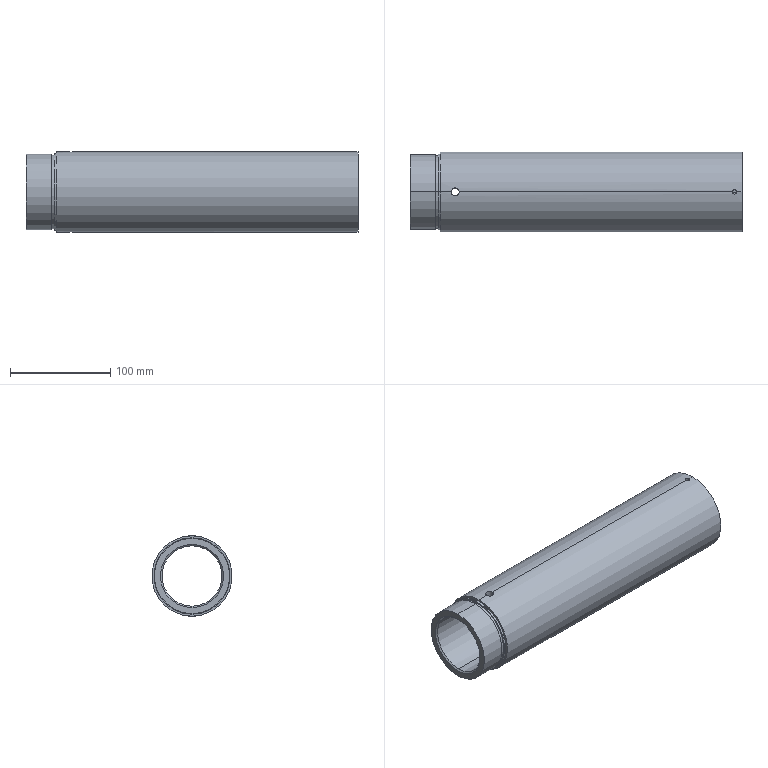Part | SolidWorks | features ICE 3, Chamfer 2, HoleWzd 1, Revolution 1 | 1 solid | 28 faces | box 330.5 x 80 x 80 mm | volume 682443 mm3 | cylinder 18 | plane 6 | cone 4 | commonest cylinder face diameters 8 x4 4.2 x2 60 x2 65 x2 73 x2 75 x2
STEP:
#1=CARTESIAN_POINT('',(320.9,0.,40.));
#2=VERTEX_POINT('',#1);
#3=CARTESIAN_POINT('',(325.1,0.,40.));
#4=VERTEX_POINT('',#3);
#5=CARTESIAN_POINT('',(320.9,0.,40.));
#6=CARTESIAN_POINT('',(320.9,-0.1388,40.));
#7=CARTESIAN_POINT('',(320.914,-0.2752,39.999));
#8=CARTESIAN_POINT('',(320.967,-0.5437,39.997));
#9=CARTESIAN_POINT('',(321.007,-0.6771,39.994));
#10=CARTESIAN_POINT('',(321.113,-0.9314,39.989));
#11=CARTESIAN_POINT('',(321.177,-1.052,39.986));
#12=CARTESIAN_POINT('',(321.33,-1.28,39.98));
#13=CARTESIAN_POINT('',(321.418,-1.388,39.976));
#14=CARTESIAN_POINT('',(321.709,-1.679,39.965));
#15=CARTESIAN_POINT('',(321.943,-1.835,39.958));
#16=CARTESIAN_POINT('',(322.449,-2.045,39.948));
#17=CARTESIAN_POINT('',(322.725,-2.1,39.945));
#18=CARTESIAN_POINT('',(323.136,-2.1,39.945));
#19=CARTESIAN_POINT('',(323.275,-2.086,39.946));
#20=CARTESIAN_POINT('',(323.545,-2.033,39.948));
#21=CARTESIAN_POINT('',(323.676,-1.993,39.95));
#22=CARTESIAN_POINT('',(323.93,-1.888,39.955));
#23=CARTESIAN_POINT('',(324.053,-1.822,39.959));
#24=CARTESIAN_POINT('',(324.28,-1.67,39.965));
#25=CARTESIAN_POINT('',(324.387,-1.583,39.969));
#26=CARTESIAN_POINT('',(324.583,-1.387,39.976));
#27=CARTESIAN_POINT('',(324.67,-1.281,39.98));
#28=CARTESIAN_POINT('',(324.822,-1.054,39.986));
#29=CARTESIAN_POINT('',(324.887,-0.9308,39.989));
#30=CARTESIAN_POINT('',(324.993,-0.6763,39.994));
#31=CARTESIAN_POINT('',(325.033,-0.5454,39.997));
#32=CARTESIAN_POINT('',(325.086,-0.2763,39.999));
#33=CARTESIAN_POINT('',(325.1,-0.1371,40.));
#34=CARTESIAN_POINT('',(325.1,0.,40.));
#35=B_SPLINE_CURVE_WITH_KNOTS('',3,(#5,#6,#7,#8,#9,#10,#11,#12,#13,#14,#15,#16,#17,#18,#19,#20,#21,#22,#23,#24,#25,#26,#27,#28,#29,#30,#31,#32,#33,#34),.UNSPECIFIED.,.F.,.F.,(4,2,2,2,2,2,2,2,2,2,2,2,2,2,4),(0.,0.0004104,0.0008208,0.001231,0.001642,0.002463,0.003283,0.003694,0.004104,0.004515,0.004925,0.005335,0.005746,0.006156,0.006567),.UNSPECIFIED.);
#36=EDGE_CURVE('',#2,#4,#35,.T.);
#37=ORIENTED_EDGE('',*,*,#36,.T.);
#38=CARTESIAN_POINT('',(325.1,0.,32.5));
#39=VERTEX_POINT('',#38);
#40=CARTESIAN_POINT('',(325.1,0.,0.));
#41=DIRECTION('',(0.,0.,-1.));
#42=VECTOR('',#41,1000.);
#43=LINE('',#40,#42);
#44=EDGE_CURVE('',#4,#39,#43,.T.);
#45=ORIENTED_EDGE('',*,*,#44,.T.);
#46=CARTESIAN_POINT('',(320.9,0.,32.5));
#47=VERTEX_POINT('',#46);
#48=CARTESIAN_POINT('',(320.9,0.,32.5));
#49=CARTESIAN_POINT('',(320.9,-0.1388,32.5));
#50=CARTESIAN_POINT('',(320.914,-0.2753,32.499));
#51=CARTESIAN_POINT('',(320.967,-0.5437,32.496));
#52=CARTESIAN_POINT('',(321.007,-0.6771,32.493));
#53=CARTESIAN_POINT('',(321.113,-0.9314,32.487));
#54=CARTESIAN_POINT('',(321.177,-1.052,32.483));
#55=CARTESIAN_POINT('',(321.33,-1.28,32.475));
#56=CARTESIAN_POINT('',(321.418,-1.388,32.47));
#57=CARTESIAN_POINT('',(321.709,-1.679,32.457));
#58=CARTESIAN_POINT('',(321.943,-1.835,32.448));
#59=CARTESIAN_POINT('',(322.449,-2.045,32.436));
#60=CARTESIAN_POINT('',(322.725,-2.1,32.432));
#61=CARTESIAN_POINT('',(323.136,-2.1,32.432));
#62=CARTESIAN_POINT('',(323.275,-2.086,32.433));
#63=CARTESIAN_POINT('',(323.545,-2.033,32.436));
#64=CARTESIAN_POINT('',(323.676,-1.993,32.439));
#65=CARTESIAN_POINT('',(323.93,-1.888,32.445));
#66=CARTESIAN_POINT('',(324.053,-1.822,32.449));
#67=CARTESIAN_POINT('',(324.281,-1.67,32.457));
#68=CARTESIAN_POINT('',(324.387,-1.583,32.462));
#69=CARTESIAN_POINT('',(324.583,-1.387,32.471));
#70=CARTESIAN_POINT('',(324.67,-1.281,32.475));
#71=CARTESIAN_POINT('',(324.822,-1.054,32.483));
#72=CARTESIAN_POINT('',(324.887,-0.9308,32.487));
#73=CARTESIAN_POINT('',(324.993,-0.6764,32.493));
#74=CARTESIAN_POINT('',(325.033,-0.5455,32.496));
#75=CARTESIAN_POINT('',(325.086,-0.2763,32.499));
#76=CARTESIAN_POINT('',(325.1,-0.1371,32.5));
#77=CARTESIAN_POINT('',(325.1,0.,32.5));
#78=B_SPLINE_CURVE_WITH_KNOTS('',3,(#48,#49,#50,#51,#52,#53,#54,#55,#56,#57,#58,#59,#60,#61,#62,#63,#64,#65,#66,#67,#68,#69,#70,#71,#72,#73,#74,#75,#76,#77),.UNSPECIFIED.,.F.,.F.,(4,2,2,2,2,2,2,2,2,2,2,2,2,2,4),(0.,0.0004105,0.0008209,0.001231,0.001642,0.002463,0.003284,0.003694,0.004105,0.004515,0.004925,0.005336,0.005746,0.006157,0.006567),.UNSPECIFIED.);
#79=EDGE_CURVE('',#47,#39,#78,.T.);
#80=ORIENTED_EDGE('',*,*,#79,.F.);
#81=CARTESIAN_POINT('',(320.9,0.,0.));
#82=DIRECTION('',(0.,0.,-1.));
#83=VECTOR('',#82,1000.);
#84=LINE('',#81,#83);
#85=EDGE_CURVE('',#2,#47,#84,.T.);
#86=ORIENTED_EDGE('',*,*,#85,.F.);
#87=EDGE_LOOP('',(#37,#45,#80,#86));
#88=FACE_OUTER_BOUND('',#87,.T.);
#89=CARTESIAN_POINT('',(323.,0.,0.));
#90=DIRECTION('',(0.,0.,-1.));
#91=DIRECTION('',(-1.,0.,0.));
#92=AXIS2_PLACEMENT_3D('',#89,#90,#91);
#93=CYLINDRICAL_SURFACE('',#92,2.1);
#94=ADVANCED_FACE('',(#88),#93,.F.);
#95=CARTESIAN_POINT('',(49.,0.,-40.));
#96=VERTEX_POINT('',#95);
#97=CARTESIAN_POINT('',(41.,0.,-40.));
#98=VERTEX_POINT('',#97);
#99=CARTESIAN_POINT('',(49.,0.,-40.));
#100=CARTESIAN_POINT('',(49.,-0.2645,-40.));
#101=CARTESIAN_POINT('',(48.974,-0.5245,-39.997));
#102=CARTESIAN_POINT('',(48.872,-1.036,-39.987));
#103=CARTESIAN_POINT('',(48.795,-1.29,-39.98));
#104=CARTESIAN_POINT('',(48.594,-1.774,-39.961));
#105=CARTESIAN_POINT('',(48.472,-2.004,-39.95));
#106=CARTESIAN_POINT('',(48.181,-2.439,-39.926));
#107=CARTESIAN_POINT('',(48.012,-2.645,-39.913));
#108=CARTESIAN_POINT('',(47.643,-3.013,-39.887));
#109=CARTESIAN_POINT('',(47.442,-3.179,-39.874));
#110=CARTESIAN_POINT('',(47.005,-3.471,-39.849));
#111=CARTESIAN_POINT('',(46.772,-3.595,-39.838));
#112=CARTESIAN_POINT('',(46.291,-3.795,-39.82));
#113=CARTESIAN_POINT('',(46.039,-3.872,-39.812));
#114=CARTESIAN_POINT('',(45.522,-3.974,-39.802));
#115=CARTESIAN_POINT('',(45.263,-4.,-39.8));
#116=CARTESIAN_POINT('',(44.74,-4.,-39.799));
#117=CARTESIAN_POINT('',(44.475,-3.974,-39.802));
#118=CARTESIAN_POINT('',(43.962,-3.872,-39.812));
#119=CARTESIAN_POINT('',(43.713,-3.796,-39.82));
#120=CARTESIAN_POINT('',(43.228,-3.596,-39.838));
#121=CARTESIAN_POINT('',(42.994,-3.47,-39.849));
#122=CARTESIAN_POINT('',(42.561,-3.181,-39.874));
#123=CARTESIAN_POINT('',(42.359,-3.016,-39.887));
#124=CARTESIAN_POINT('',(41.985,-2.642,-39.913));
#125=CARTESIAN_POINT('',(41.82,-2.44,-39.926));
#126=CARTESIAN_POINT('',(41.53,-2.007,-39.95));
#127=CARTESIAN_POINT('',(41.405,-1.773,-39.961));
#128=CARTESIAN_POINT('',(41.204,-1.289,-39.98));
#129=CARTESIAN_POINT('',(41.129,-1.039,-39.987));
#130=CARTESIAN_POINT('',(41.026,-0.5264,-39.997));
#131=CARTESIAN_POINT('',(41.,-0.2611,-40.));
#132=CARTESIAN_POINT('',(41.,0.,-40.));
#133=B_SPLINE_CURVE_WITH_KNOTS('',3,(#99,#100,#101,#102,#103,#104,#105,#106,#107,#108,#109,#110,#111,#112,#113,#114,#115,#116,#117,#118,#119,#120,#121,#122,#123,#124,#125,#126,#127,#128,#129,#130,#131,#132),.UNSPECIFIED.,.F.,.F.,(4,2,2,2,2,2,2,2,2,2,2,2,2,2,2,2,4),(0.,0.0007821,0.001564,0.002346,0.003128,0.003911,0.004693,0.005475,0.006257,0.007039,0.007821,0.008603,0.009385,0.01017,0.01095,0.01173,0.01251),.UNSPECIFIED.);
#134=EDGE_CURVE('',#96,#98,#133,.T.);
#135=ORIENTED_EDGE('',*,*,#134,.T.);
#136=CARTESIAN_POINT('',(41.,0.,-30.));
#137=VERTEX_POINT('',#136);
#138=CARTESIAN_POINT('',(41.,0.,-40.));
#139=DIRECTION('',(0.,0.,1.));
#140=VECTOR('',#139,1000.);
#141=LINE('',#138,#140);
#142=EDGE_CURVE('',#98,#137,#141,.T.);
#143=ORIENTED_EDGE('',*,*,#142,.T.);
#144=CARTESIAN_POINT('',(49.,0.,-30.));
#145=VERTEX_POINT('',#144);
#146=CARTESIAN_POINT('',(49.,0.,-30.));
#147=CARTESIAN_POINT('',(49.,-0.2611,-30.));
#148=CARTESIAN_POINT('',(48.975,-0.5209,-29.997));
#149=CARTESIAN_POINT('',(48.872,-1.038,-29.983));
#150=CARTESIAN_POINT('',(48.795,-1.29,-29.973));
#151=CARTESIAN_POINT('',(48.596,-1.771,-29.949));
#152=CARTESIAN_POINT('',(48.472,-2.004,-29.934));
#153=CARTESIAN_POINT('',(48.18,-2.441,-29.901));
#154=CARTESIAN_POINT('',(48.015,-2.642,-29.884));
#155=CARTESIAN_POINT('',(47.646,-3.011,-29.849));
#156=CARTESIAN_POINT('',(47.441,-3.18,-29.831));
#157=CARTESIAN_POINT('',(47.007,-3.47,-29.799));
#158=CARTESIAN_POINT('',(46.777,-3.593,-29.784));
#159=CARTESIAN_POINT('',(46.293,-3.794,-29.759));
#160=CARTESIAN_POINT('',(46.039,-3.872,-29.749));
#161=CARTESIAN_POINT('',(45.528,-3.974,-29.736));
#162=CARTESIAN_POINT('',(45.267,-4.,-29.732));
#163=CARTESIAN_POINT('',(44.738,-4.,-29.732));
#164=CARTESIAN_POINT('',(44.478,-3.974,-29.736));
#165=CARTESIAN_POINT('',(43.967,-3.873,-29.749));
#166=CARTESIAN_POINT('',(43.712,-3.796,-29.759));
#167=CARTESIAN_POINT('',(43.228,-3.596,-29.784));
#168=CARTESIAN_POINT('',(42.998,-3.473,-29.799));
#169=CARTESIAN_POINT('',(42.563,-3.183,-29.831));
#170=CARTESIAN_POINT('',(42.358,-3.014,-29.849));
#171=CARTESIAN_POINT('',(41.989,-2.646,-29.884));
#172=CARTESIAN_POINT('',(41.824,-2.445,-29.901));
#173=CARTESIAN_POINT('',(41.531,-2.008,-29.934));
#174=CARTESIAN_POINT('',(41.407,-1.776,-29.948));
#175=CARTESIAN_POINT('',(41.207,-1.295,-29.973));
#176=CARTESIAN_POINT('',(41.129,-1.043,-29.983));
#177=CARTESIAN_POINT('',(41.026,-0.526,-29.997));
#178=CARTESIAN_POINT('',(41.,-0.2645,-30.));
#179=CARTESIAN_POINT('',(41.,0.,-30.));
#180=B_SPLINE_CURVE_WITH_KNOTS('',3,(#146,#147,#148,#149,#150,#151,#152,#153,#154,#155,#156,#157,#158,#159,#160,#161,#162,#163,#164,#165,#166,#167,#168,#169,#170,#171,#172,#173,#174,#175,#176,#177,#178,#179),.UNSPECIFIED.,.F.,.F.,(4,2,2,2,2,2,2,2,2,2,2,2,2,2,2,2,4),(0.01252,0.0133,0.01408,0.01487,0.01565,0.01643,0.01721,0.018,0.01878,0.01956,0.02034,0.02113,0.02191,0.02269,0.02347,0.02425,0.02504),.UNSPECIFIED.);
#181=EDGE_CURVE('',#145,#137,#180,.T.);
#182=ORIENTED_EDGE('',*,*,#181,.F.);
#183=CARTESIAN_POINT('',(49.,0.,-40.));
#184=DIRECTION('',(0.,0.,1.));
#185=VECTOR('',#184,1000.);
#186=LINE('',#183,#185);
#187=EDGE_CURVE('',#96,#145,#186,.T.);
#188=ORIENTED_EDGE('',*,*,#187,.F.);
#189=EDGE_LOOP('',(#135,#143,#182,#188));
#190=FACE_OUTER_BOUND('',#189,.T.);
#191=CARTESIAN_POINT('',(45.,0.,-40.));
#192=DIRECTION('',(0.,0.,1.));
#193=DIRECTION('',(1.,0.,0.));
#194=AXIS2_PLACEMENT_3D('',#191,#192,#193);
#195=CYLINDRICAL_SURFACE('',#194,4.);
#196=ADVANCED_FACE('',(#190),#195,.F.);
#197=CARTESIAN_POINT('',(41.,0.,30.));
#198=VERTEX_POINT('',#197);
#199=CARTESIAN_POINT('',(49.,0.,30.));
#200=VERTEX_POINT('',#199);
#201=CARTESIAN_POINT('',(41.,0.,30.));
#202=CARTESIAN_POINT('',(41.,-0.2611,30.));
#203=CARTESIAN_POINT('',(41.025,-0.5209,29.997));
#204=CARTESIAN_POINT('',(41.128,-1.038,29.983));
#205=CARTESIAN_POINT('',(41.205,-1.29,29.973));
#206=CARTESIAN_POINT('',(41.404,-1.771,29.949));
#207=CARTESIAN_POINT('',(41.528,-2.004,29.934));
#208=CARTESIAN_POINT('',(41.82,-2.441,29.901));
#209=CARTESIAN_POINT('',(41.985,-2.642,29.884));
#210=CARTESIAN_POINT('',(42.354,-3.011,29.849));
#211=CARTESIAN_POINT('',(42.559,-3.18,29.831));
#212=CARTESIAN_POINT('',(42.993,-3.47,29.799));
#213=CARTESIAN_POINT('',(43.223,-3.593,29.784));
#214=CARTESIAN_POINT('',(43.707,-3.794,29.759));
#215=CARTESIAN_POINT('',(43.961,-3.872,29.749));
#216=CARTESIAN_POINT('',(44.472,-3.974,29.736));
#217=CARTESIAN_POINT('',(44.733,-4.,29.732));
#218=CARTESIAN_POINT('',(45.262,-4.,29.732));
#219=CARTESIAN_POINT('',(45.522,-3.974,29.736));
#220=CARTESIAN_POINT('',(46.033,-3.873,29.749));
#221=CARTESIAN_POINT('',(46.288,-3.796,29.759));
#222=CARTESIAN_POINT('',(46.772,-3.596,29.784));
#223=CARTESIAN_POINT('',(47.002,-3.473,29.799));
#224=CARTESIAN_POINT('',(47.437,-3.183,29.831));
#225=CARTESIAN_POINT('',(47.642,-3.014,29.849));
#226=CARTESIAN_POINT('',(48.011,-2.646,29.884));
#227=CARTESIAN_POINT('',(48.176,-2.445,29.901));
#228=CARTESIAN_POINT('',(48.469,-2.008,29.934));
#229=CARTESIAN_POINT('',(48.593,-1.776,29.948));
#230=CARTESIAN_POINT('',(48.793,-1.295,29.973));
#231=CARTESIAN_POINT('',(48.871,-1.043,29.983));
#232=CARTESIAN_POINT('',(48.974,-0.526,29.997));
#233=CARTESIAN_POINT('',(49.,-0.2645,30.));
#234=CARTESIAN_POINT('',(49.,0.,30.));
#235=B_SPLINE_CURVE_WITH_KNOTS('',3,(#201,#202,#203,#204,#205,#206,#207,#208,#209,#210,#211,#212,#213,#214,#215,#216,#217,#218,#219,#220,#221,#222,#223,#224,#225,#226,#227,#228,#229,#230,#231,#232,#233,#234),.UNSPECIFIED.,.F.,.F.,(4,2,2,2,2,2,2,2,2,2,2,2,2,2,2,2,4),(0.01252,0.0133,0.01408,0.01487,0.01565,0.01643,0.01721,0.018,0.01878,0.01956,0.02034,0.02113,0.02191,0.02269,0.02347,0.02425,0.02504),.UNSPECIFIED.);
#236=EDGE_CURVE('',#198,#200,#235,.T.);
#237=ORIENTED_EDGE('',*,*,#236,.F.);
#238=CARTESIAN_POINT('',(41.,0.,40.));
#239=VERTEX_POINT('',#238);
#240=CARTESIAN_POINT('',(41.,0.,-40.));
#241=DIRECTION('',(0.,0.,1.));
#242=VECTOR('',#241,1000.);
#243=LINE('',#240,#242);
#244=EDGE_CURVE('',#198,#239,#243,.T.);
#245=ORIENTED_EDGE('',*,*,#244,.T.);
#246=CARTESIAN_POINT('',(49.,0.,40.));
#247=VERTEX_POINT('',#246);
#248=CARTESIAN_POINT('',(41.,0.,40.));
#249=CARTESIAN_POINT('',(41.,-0.2611,40.));
#250=CARTESIAN_POINT('',(41.025,-0.5207,39.997));
#251=CARTESIAN_POINT('',(41.128,-1.037,39.987));
#252=CARTESIAN_POINT('',(41.205,-1.289,39.98));
#253=CARTESIAN_POINT('',(41.404,-1.771,39.962));
#254=CARTESIAN_POINT('',(41.528,-2.003,39.95));
#255=CARTESIAN_POINT('',(41.82,-2.441,39.926));
#256=CARTESIAN_POINT('',(41.985,-2.642,39.913));
#257=CARTESIAN_POINT('',(42.354,-3.011,39.887));
#258=CARTESIAN_POINT('',(42.559,-3.18,39.874));
#259=CARTESIAN_POINT('',(42.994,-3.47,39.849));
#260=CARTESIAN_POINT('',(43.223,-3.593,39.838));
#261=CARTESIAN_POINT('',(43.707,-3.794,39.82));
#262=CARTESIAN_POINT('',(43.962,-3.872,39.812));
#263=CARTESIAN_POINT('',(44.473,-3.974,39.802));
#264=CARTESIAN_POINT('',(44.733,-4.,39.8));
#265=CARTESIAN_POINT('',(45.261,-4.,39.799));
#266=CARTESIAN_POINT('',(45.522,-3.974,39.802));
#267=CARTESIAN_POINT('',(46.033,-3.873,39.812));
#268=CARTESIAN_POINT('',(46.287,-3.796,39.82));
#269=CARTESIAN_POINT('',(46.772,-3.596,39.838));
#270=CARTESIAN_POINT('',(47.001,-3.473,39.849));
#271=CARTESIAN_POINT('',(47.436,-3.183,39.873));
#272=CARTESIAN_POINT('',(47.642,-3.015,39.887));
#273=CARTESIAN_POINT('',(48.011,-2.646,39.913));
#274=CARTESIAN_POINT('',(48.177,-2.445,39.926));
#275=CARTESIAN_POINT('',(48.469,-2.008,39.95));
#276=CARTESIAN_POINT('',(48.594,-1.776,39.961));
#277=CARTESIAN_POINT('',(48.794,-1.295,39.98));
#278=CARTESIAN_POINT('',(48.871,-1.043,39.987));
#279=CARTESIAN_POINT('',(48.974,-0.5259,39.997));
#280=CARTESIAN_POINT('',(49.,-0.2644,40.));
#281=CARTESIAN_POINT('',(49.,0.,40.));
#282=B_SPLINE_CURVE_WITH_KNOTS('',3,(#248,#249,#250,#251,#252,#253,#254,#255,#256,#257,#258,#259,#260,#261,#262,#263,#264,#265,#266,#267,#268,#269,#270,#271,#272,#273,#274,#275,#276,#277,#278,#279,#280,#281),.UNSPECIFIED.,.F.,.F.,(4,2,2,2,2,2,2,2,2,2,2,2,2,2,2,2,4),(0.01251,0.0133,0.01408,0.01486,0.01564,0.01642,0.01721,0.01799,0.01877,0.01955,0.02033,0.02111,0.0219,0.02268,0.02346,0.02424,0.02502),.UNSPECIFIED.);
#283=EDGE_CURVE('',#239,#247,#282,.T.);
#284=ORIENTED_EDGE('',*,*,#283,.T.);
#285=CARTESIAN_POINT('',(49.,0.,-40.));
#286=DIRECTION('',(0.,0.,1.));
#287=VECTOR('',#286,1000.);
#288=LINE('',#285,#287);
#289=EDGE_CURVE('',#200,#247,#288,.T.);
#290=ORIENTED_EDGE('',*,*,#289,.F.);
#291=EDGE_LOOP('',(#237,#245,#284,#290));
#292=FACE_OUTER_BOUND('',#291,.T.);
#293=CARTESIAN_POINT('',(45.,0.,-40.));
#294=DIRECTION('',(0.,0.,1.));
#295=DIRECTION('',(1.,0.,0.));
#296=AXIS2_PLACEMENT_3D('',#293,#294,#295);
#297=CYLINDRICAL_SURFACE('',#296,4.);
#298=ADVANCED_FACE('',(#292),#297,.F.);
#299=CARTESIAN_POINT('',(1.5,0.,-30.));
#300=VERTEX_POINT('',#299);
#301=CARTESIAN_POINT('',(1.5,0.,30.));
#302=VERTEX_POINT('',#301);
#303=CARTESIAN_POINT('',(1.5,0.,0.));
#304=DIRECTION('',(-1.,0.,0.));
#305=DIRECTION('',(0.,0.,1.));
#306=AXIS2_PLACEMENT_3D('',#303,#304,#305);
#307=CIRCLE('',#306,30.);
#308=EDGE_CURVE('',#300,#302,#307,.T.);
#309=ORIENTED_EDGE('',*,*,#308,.F.);
#310=CARTESIAN_POINT('',(0.,0.,-31.5));
#311=VERTEX_POINT('',#310);
#312=CARTESIAN_POINT('',(0.,0.,-31.5));
#313=DIRECTION('',(-0.7071,0.,-0.7071));
#314=VECTOR('',#313,1000.);
#315=LINE('',#312,#314);
#316=EDGE_CURVE('',#300,#311,#315,.T.);
#317=ORIENTED_EDGE('',*,*,#316,.T.);
#318=CARTESIAN_POINT('',(0.,0.,31.5));
#319=VERTEX_POINT('',#318);
#320=CARTESIAN_POINT('',(0.,0.,0.));
#321=DIRECTION('',(1.,0.,0.));
#322=DIRECTION('',(0.,0.,1.));
#323=AXIS2_PLACEMENT_3D('',#320,#321,#322);
#324=CIRCLE('',#323,31.5);
#325=EDGE_CURVE('',#319,#311,#324,.T.);
#326=ORIENTED_EDGE('',*,*,#325,.F.);
#327=CARTESIAN_POINT('',(0.,0.,31.5));
#328=DIRECTION('',(-0.7071,0.,0.7071));
#329=VECTOR('',#328,1000.);
#330=LINE('',#327,#329);
#331=EDGE_CURVE('',#302,#319,#330,.T.);
#332=ORIENTED_EDGE('',*,*,#331,.F.);
#333=EDGE_LOOP('',(#309,#317,#326,#332));
#334=FACE_OUTER_BOUND('',#333,.T.);
#335=CARTESIAN_POINT('',(0.,0.,0.));
#336=DIRECTION('',(-1.,0.,0.));
#337=DIRECTION('',(0.,0.,1.));
#338=AXIS2_PLACEMENT_3D('',#335,#336,#337);
#339=CONICAL_SURFACE('',#338,31.5,0.7854);
#340=ADVANCED_FACE('',(#334),#339,.F.);
#341=CARTESIAN_POINT('',(280.5,0.,31.));
#342=VERTEX_POINT('',#341);
#343=CARTESIAN_POINT('',(280.5,0.,-31.));
#344=VERTEX_POINT('',#343);
#345=CARTESIAN_POINT('',(280.5,0.,0.));
#346=DIRECTION('',(1.,0.,0.));
#347=DIRECTION('',(0.,0.,-1.));
#348=AXIS2_PLACEMENT_3D('',#345,#346,#347);
#349=CIRCLE('',#348,31.);
#350=EDGE_CURVE('',#342,#344,#349,.T.);
#351=ORIENTED_EDGE('',*,*,#350,.F.);
#352=CARTESIAN_POINT('',(282.,0.,32.5));
#353=VERTEX_POINT('',#352);
#354=CARTESIAN_POINT('',(280.5,0.,31.));
#355=DIRECTION('',(0.7071,0.,0.7071));
#356=VECTOR('',#355,1000.);
#357=LINE('',#354,#356);
#358=EDGE_CURVE('',#342,#353,#357,.T.);
#359=ORIENTED_EDGE('',*,*,#358,.T.);
#360=CARTESIAN_POINT('',(282.,0.,-32.5));
#361=VERTEX_POINT('',#360);
#362=CARTESIAN_POINT('',(282.,0.,0.));
#363=DIRECTION('',(-1.,0.,0.));
#364=DIRECTION('',(0.,0.,-1.));
#365=AXIS2_PLACEMENT_3D('',#362,#363,#364);
#366=CIRCLE('',#365,32.5);
#367=EDGE_CURVE('',#361,#353,#366,.T.);
#368=ORIENTED_EDGE('',*,*,#367,.F.);
#369=CARTESIAN_POINT('',(280.5,0.,-31.));
#370=DIRECTION('',(0.7071,0.,-0.7071));
#371=VECTOR('',#370,1000.);
#372=LINE('',#369,#371);
#373=EDGE_CURVE('',#344,#361,#372,.T.);
#374=ORIENTED_EDGE('',*,*,#373,.F.);
#375=EDGE_LOOP('',(#351,#359,#368,#374));
#376=FACE_OUTER_BOUND('',#375,.T.);
#377=CARTESIAN_POINT('',(280.5,0.,0.));
#378=DIRECTION('',(1.,0.,0.));
#379=DIRECTION('',(0.,0.,-1.));
#380=AXIS2_PLACEMENT_3D('',#377,#378,#379);
#381=CONICAL_SURFACE('',#380,31.,0.7854);
#382=ADVANCED_FACE('',(#376),#381,.F.);
#383=ORIENTED_EDGE('',*,*,#308,.T.);
#384=CARTESIAN_POINT('',(0.,0.,30.));
#385=DIRECTION('',(1.,0.,0.));
#386=VECTOR('',#385,1000.);
#387=LINE('',#384,#386);
#388=EDGE_CURVE('',#302,#198,#387,.T.);
#389=ORIENTED_EDGE('',*,*,#388,.T.);
#390=ORIENTED_EDGE('',*,*,#236,.T.);
#391=CARTESIAN_POINT('',(280.5,0.,30.));
#392=VERTEX_POINT('',#391);
#393=CARTESIAN_POINT('',(0.,0.,30.));
#394=DIRECTION('',(1.,0.,0.));
#395=VECTOR('',#394,1000.);
#396=LINE('',#393,#395);
#397=EDGE_CURVE('',#200,#392,#396,.T.);
#398=ORIENTED_EDGE('',*,*,#397,.T.);
#399=CARTESIAN_POINT('',(280.5,0.,-30.));
#400=VERTEX_POINT('',#399);
#401=CARTESIAN_POINT('',(280.5,0.,0.));
#402=DIRECTION('',(1.,0.,0.));
#403=DIRECTION('',(0.,0.,-1.));
#404=AXIS2_PLACEMENT_3D('',#401,#402,#403);
#405=CIRCLE('',#404,30.);
#406=EDGE_CURVE('',#392,#400,#405,.T.);
#407=ORIENTED_EDGE('',*,*,#406,.T.);
#408=CARTESIAN_POINT('',(0.,0.,-30.));
#409=DIRECTION('',(1.,0.,0.));
#410=VECTOR('',#409,1000.);
#411=LINE('',#408,#410);
#412=EDGE_CURVE('',#145,#400,#411,.T.);
#413=ORIENTED_EDGE('',*,*,#412,.F.);
#414=ORIENTED_EDGE('',*,*,#181,.T.);
#415=CARTESIAN_POINT('',(0.,0.,-30.));
#416=DIRECTION('',(1.,0.,0.));
#417=VECTOR('',#416,1000.);
#418=LINE('',#415,#417);
#419=EDGE_CURVE('',#300,#137,#418,.T.);
#420=ORIENTED_EDGE('',*,*,#419,.F.);
#421=EDGE_LOOP('',(#383,#389,#390,#398,#407,#413,#414,#420));
#422=FACE_OUTER_BOUND('',#421,.T.);
#423=CARTESIAN_POINT('',(0.,0.,0.));
#424=DIRECTION('',(1.,0.,0.));
#425=DIRECTION('',(0.,0.,-1.));
#426=AXIS2_PLACEMENT_3D('',#423,#424,#425);
#427=CYLINDRICAL_SURFACE('',#426,30.);
#428=ADVANCED_FACE('',(#422),#427,.F.);
#429=ORIENTED_EDGE('',*,*,#367,.T.);
#430=CARTESIAN_POINT('',(280.5,0.,32.5));
#431=DIRECTION('',(1.,0.,0.));
#432=VECTOR('',#431,1000.);
#433=LINE('',#430,#432);
#434=EDGE_CURVE('',#353,#47,#433,.T.);
#435=ORIENTED_EDGE('',*,*,#434,.T.);
#436=ORIENTED_EDGE('',*,*,#79,.T.);
#437=CARTESIAN_POINT('',(330.5,0.,32.5));
#438=VERTEX_POINT('',#437);
#439=CARTESIAN_POINT('',(280.5,0.,32.5));
#440=DIRECTION('',(1.,0.,0.));
#441=VECTOR('',#440,1000.);
#442=LINE('',#439,#441);
#443=EDGE_CURVE('',#39,#438,#442,.T.);
#444=ORIENTED_EDGE('',*,*,#443,.T.);
#445=CARTESIAN_POINT('',(330.5,0.,-32.5));
#446=VERTEX_POINT('',#445);
#447=CARTESIAN_POINT('',(330.5,0.,0.));
#448=DIRECTION('',(1.,0.,0.));
#449=DIRECTION('',(0.,0.,-1.));
#450=AXIS2_PLACEMENT_3D('',#447,#448,#449);
#451=CIRCLE('',#450,32.5);
#452=EDGE_CURVE('',#438,#446,#451,.T.);
#453=ORIENTED_EDGE('',*,*,#452,.T.);
#454=CARTESIAN_POINT('',(280.5,0.,-32.5));
#455=DIRECTION('',(1.,0.,0.));
#456=VECTOR('',#455,1000.);
#457=LINE('',#454,#456);
#458=EDGE_CURVE('',#361,#446,#457,.T.);
#459=ORIENTED_EDGE('',*,*,#458,.F.);
#460=EDGE_LOOP('',(#429,#435,#436,#444,#453,#459));
#461=FACE_OUTER_BOUND('',#460,.T.);
#462=CARTESIAN_POINT('',(280.5,0.,0.));
#463=DIRECTION('',(1.,0.,0.));
#464=DIRECTION('',(0.,0.,-1.));
#465=AXIS2_PLACEMENT_3D('',#462,#463,#464);
#466=CYLINDRICAL_SURFACE('',#465,32.5);
#467=ADVANCED_FACE('',(#461),#466,.F.);
#468=CARTESIAN_POINT('',(30.,0.,-40.));
#469=VERTEX_POINT('',#468);
#470=CARTESIAN_POINT('',(30.,0.,40.));
#471=VERTEX_POINT('',#470);
#472=CARTESIAN_POINT('',(30.,0.,0.));
#473=DIRECTION('',(1.,0.,0.));
#474=DIRECTION('',(0.,0.,-1.));
#475=AXIS2_PLACEMENT_3D('',#472,#473,#474);
#476=CIRCLE('',#475,40.);
#477=EDGE_CURVE('',#469,#471,#476,.T.);
#478=ORIENTED_EDGE('',*,*,#477,.T.);
#479=CARTESIAN_POINT('',(0.,0.,40.));
#480=DIRECTION('',(1.,0.,0.));
#481=VECTOR('',#480,1000.);
#482=LINE('',#479,#481);
#483=EDGE_CURVE('',#471,#239,#482,.T.);
#484=ORIENTED_EDGE('',*,*,#483,.T.);
#485=CARTESIAN_POINT('',(49.,0.,40.));
#486=CARTESIAN_POINT('',(49.,0.2645,40.));
#487=CARTESIAN_POINT('',(48.974,0.5245,39.997));
#488=CARTESIAN_POINT('',(48.872,1.036,39.987));
#489=CARTESIAN_POINT('',(48.795,1.29,39.98));
#490=CARTESIAN_POINT('',(48.594,1.774,39.961));
#491=CARTESIAN_POINT('',(48.472,2.004,39.95));
#492=CARTESIAN_POINT('',(48.181,2.439,39.926));
#493=CARTESIAN_POINT('',(48.012,2.645,39.913));
#494=CARTESIAN_POINT('',(47.643,3.013,39.887));
#495=CARTESIAN_POINT('',(47.442,3.179,39.874));
#496=CARTESIAN_POINT('',(47.005,3.471,39.849));
#497=CARTESIAN_POINT('',(46.772,3.595,39.838));
#498=CARTESIAN_POINT('',(46.291,3.795,39.82));
#499=CARTESIAN_POINT('',(46.039,3.872,39.812));
#500=CARTESIAN_POINT('',(45.522,3.974,39.802));
#501=CARTESIAN_POINT('',(45.263,4.,39.8));
#502=CARTESIAN_POINT('',(44.74,4.,39.799));
#503=CARTESIAN_POINT('',(44.475,3.974,39.802));
#504=CARTESIAN_POINT('',(43.962,3.872,39.812));
#505=CARTESIAN_POINT('',(43.713,3.796,39.82));
#506=CARTESIAN_POINT('',(43.228,3.596,39.838));
#507=CARTESIAN_POINT('',(42.994,3.47,39.849));
#508=CARTESIAN_POINT('',(42.561,3.181,39.874));
#509=CARTESIAN_POINT('',(42.359,3.016,39.887));
#510=CARTESIAN_POINT('',(41.985,2.642,39.913));
#511=CARTESIAN_POINT('',(41.82,2.44,39.926));
#512=CARTESIAN_POINT('',(41.53,2.007,39.95));
#513=CARTESIAN_POINT('',(41.405,1.773,39.961));
#514=CARTESIAN_POINT('',(41.204,1.289,39.98));
#515=CARTESIAN_POINT('',(41.129,1.039,39.987));
#516=CARTESIAN_POINT('',(41.026,0.5264,39.997));
#517=CARTESIAN_POINT('',(41.,0.2611,40.));
#518=CARTESIAN_POINT('',(41.,0.,40.));
#519=B_SPLINE_CURVE_WITH_KNOTS('',3,(#485,#486,#487,#488,#489,#490,#491,#492,#493,#494,#495,#496,#497,#498,#499,#500,#501,#502,#503,#504,#505,#506,#507,#508,#509,#510,#511,#512,#513,#514,#515,#516,#517,#518),.UNSPECIFIED.,.F.,.F.,(4,2,2,2,2,2,2,2,2,2,2,2,2,2,2,2,4),(0.,0.0007821,0.001564,0.002346,0.003128,0.003911,0.004693,0.005475,0.006257,0.007039,0.007821,0.008603,0.009385,0.01017,0.01095,0.01173,0.01251),.UNSPECIFIED.);
#520=EDGE_CURVE('',#247,#239,#519,.T.);
#521=ORIENTED_EDGE('',*,*,#520,.F.);
#522=CARTESIAN_POINT('',(0.,0.,40.));
#523=DIRECTION('',(1.,0.,0.));
#524=VECTOR('',#523,1000.);
#525=LINE('',#522,#524);
#526=EDGE_CURVE('',#247,#2,#525,.T.);
#527=ORIENTED_EDGE('',*,*,#526,.T.);
#528=CARTESIAN_POINT('',(325.1,0.,40.));
#529=CARTESIAN_POINT('',(325.1,0.137,40.));
#530=CARTESIAN_POINT('',(325.087,0.2732,39.999));
#531=CARTESIAN_POINT('',(325.033,0.544,39.997));
#532=CARTESIAN_POINT('',(324.993,0.6767,39.994));
#533=CARTESIAN_POINT('',(324.836,1.056,39.987));
#534=CARTESIAN_POINT('',(324.679,1.29,39.98));
#535=CARTESIAN_POINT('',(324.389,1.581,39.969));
#536=CARTESIAN_POINT('',(324.281,1.669,39.965));
#537=CARTESIAN_POINT('',(324.053,1.822,39.959));
#538=CARTESIAN_POINT('',(323.932,1.887,39.956));
#539=CARTESIAN_POINT('',(323.679,1.992,39.95));
#540=CARTESIAN_POINT('',(323.545,2.033,39.948));
#541=CARTESIAN_POINT('',(323.277,2.086,39.946));
#542=CARTESIAN_POINT('',(323.14,2.1,39.945));
#543=CARTESIAN_POINT('',(322.863,2.1,39.945));
#544=CARTESIAN_POINT('',(322.726,2.087,39.946));
#545=CARTESIAN_POINT('',(322.458,2.033,39.948));
#546=CARTESIAN_POINT('',(322.325,1.993,39.95));
#547=CARTESIAN_POINT('',(322.07,1.888,39.955));
#548=CARTESIAN_POINT('',(321.949,1.823,39.958));
#549=CARTESIAN_POINT('',(321.721,1.671,39.965));
#550=CARTESIAN_POINT('',(321.613,1.583,39.969));
#551=CARTESIAN_POINT('',(321.419,1.389,39.976));
#552=CARTESIAN_POINT('',(321.332,1.284,39.98));
#553=CARTESIAN_POINT('',(321.179,1.054,39.986));
#554=CARTESIAN_POINT('',(321.113,0.932,39.989));
#555=CARTESIAN_POINT('',(320.956,0.5532,39.997));
#556=CARTESIAN_POINT('',(320.9,0.2775,40.));
#557=CARTESIAN_POINT('',(320.9,0.,40.));
#558=B_SPLINE_CURVE_WITH_KNOTS('',3,(#528,#529,#530,#531,#532,#533,#534,#535,#536,#537,#538,#539,#540,#541,#542,#543,#544,#545,#546,#547,#548,#549,#550,#551,#552,#553,#554,#555,#556,#557),.UNSPECIFIED.,.F.,.F.,(4,2,2,2,2,2,2,2,2,2,2,2,2,2,4),(0.006567,0.006977,0.007387,0.008208,0.008618,0.009029,0.009439,0.009849,0.01026,0.01067,0.01108,0.01149,0.0119,0.01231,0.01313),.UNSPECIFIED.);
#559=EDGE_CURVE('',#4,#2,#558,.T.);
#560=ORIENTED_EDGE('',*,*,#559,.F.);
#561=CARTESIAN_POINT('',(330.5,0.,40.));
#562=VERTEX_POINT('',#561);
#563=CARTESIAN_POINT('',(0.,0.,40.));
#564=DIRECTION('',(1.,0.,0.));
#565=VECTOR('',#564,1000.);
#566=LINE('',#563,#565);
#567=EDGE_CURVE('',#4,#562,#566,.T.);
#568=ORIENTED_EDGE('',*,*,#567,.T.);
#569=CARTESIAN_POINT('',(330.5,0.,-40.));
#570=VERTEX_POINT('',#569);
#571=CARTESIAN_POINT('',(330.5,0.,0.));
#572=DIRECTION('',(1.,0.,0.));
#573=DIRECTION('',(0.,0.,-1.));
#574=AXIS2_PLACEMENT_3D('',#571,#572,#573);
#575=CIRCLE('',#574,40.);
#576=EDGE_CURVE('',#570,#562,#575,.T.);
#577=ORIENTED_EDGE('',*,*,#576,.F.);
#578=CARTESIAN_POINT('',(0.,0.,-40.));
#579=DIRECTION('',(1.,0.,0.));
#580=VECTOR('',#579,1000.);
#581=LINE('',#578,#580);
#582=EDGE_CURVE('',#96,#570,#581,.T.);
#583=ORIENTED_EDGE('',*,*,#582,.F.);
#584=CARTESIAN_POINT('',(41.,0.,-40.));
#585=CARTESIAN_POINT('',(41.,0.2611,-40.));
#586=CARTESIAN_POINT('',(41.025,0.5207,-39.997));
#587=CARTESIAN_POINT('',(41.128,1.037,-39.987));
#588=CARTESIAN_POINT('',(41.205,1.289,-39.98));
#589=CARTESIAN_POINT('',(41.404,1.771,-39.962));
#590=CARTESIAN_POINT('',(41.528,2.003,-39.95));
#591=CARTESIAN_POINT('',(41.82,2.441,-39.926));
#592=CARTESIAN_POINT('',(41.985,2.642,-39.913));
#593=CARTESIAN_POINT('',(42.354,3.011,-39.887));
#594=CARTESIAN_POINT('',(42.559,3.18,-39.874));
#595=CARTESIAN_POINT('',(42.994,3.47,-39.849));
#596=CARTESIAN_POINT('',(43.223,3.593,-39.838));
#597=CARTESIAN_POINT('',(43.707,3.794,-39.82));
#598=CARTESIAN_POINT('',(43.962,3.872,-39.812));
#599=CARTESIAN_POINT('',(44.473,3.974,-39.802));
#600=CARTESIAN_POINT('',(44.733,4.,-39.8));
#601=CARTESIAN_POINT('',(45.261,4.,-39.799));
#602=CARTESIAN_POINT('',(45.522,3.974,-39.802));
#603=CARTESIAN_POINT('',(46.033,3.873,-39.812));
#604=CARTESIAN_POINT('',(46.287,3.796,-39.82));
#605=CARTESIAN_POINT('',(46.772,3.596,-39.838));
#606=CARTESIAN_POINT('',(47.001,3.473,-39.849));
#607=CARTESIAN_POINT('',(47.436,3.183,-39.873));
#608=CARTESIAN_POINT('',(47.642,3.015,-39.887));
#609=CARTESIAN_POINT('',(48.011,2.646,-39.913));
#610=CARTESIAN_POINT('',(48.177,2.445,-39.926));
#611=CARTESIAN_POINT('',(48.469,2.008,-39.95));
#612=CARTESIAN_POINT('',(48.594,1.776,-39.961));
#613=CARTESIAN_POINT('',(48.794,1.295,-39.98));
#614=CARTESIAN_POINT('',(48.871,1.043,-39.987));
#615=CARTESIAN_POINT('',(48.974,0.5259,-39.997));
#616=CARTESIAN_POINT('',(49.,0.2644,-40.));
#617=CARTESIAN_POINT('',(49.,0.,-40.));
#618=B_SPLINE_CURVE_WITH_KNOTS('',3,(#584,#585,#586,#587,#588,#589,#590,#591,#592,#593,#594,#595,#596,#597,#598,#599,#600,#601,#602,#603,#604,#605,#606,#607,#608,#609,#610,#611,#612,#613,#614,#615,#616,#617),.UNSPECIFIED.,.F.,.F.,(4,2,2,2,2,2,2,2,2,2,2,2,2,2,2,2,4),(0.01251,0.0133,0.01408,0.01486,0.01564,0.01642,0.01721,0.01799,0.01877,0.01955,0.02033,0.02111,0.0219,0.02268,0.02346,0.02424,0.02502),.UNSPECIFIED.);
#619=EDGE_CURVE('',#98,#96,#618,.T.);
#620=ORIENTED_EDGE('',*,*,#619,.F.);
#621=CARTESIAN_POINT('',(0.,0.,-40.));
#622=DIRECTION('',(1.,0.,0.));
#623=VECTOR('',#622,1000.);
#624=LINE('',#621,#623);
#625=EDGE_CURVE('',#469,#98,#624,.T.);
#626=ORIENTED_EDGE('',*,*,#625,.F.);
#627=EDGE_LOOP('',(#478,#484,#521,#527,#560,#568,#577,#583,#620,#626));
#628=FACE_OUTER_BOUND('',#627,.T.);
#629=CARTESIAN_POINT('',(0.,0.,0.));
#630=DIRECTION('',(1.,0.,0.));
#631=DIRECTION('',(0.,0.,-1.));
#632=AXIS2_PLACEMENT_3D('',#629,#630,#631);
#633=CYLINDRICAL_SURFACE('',#632,40.);
#634=ADVANCED_FACE('',(#628),#633,.T.);
#635=CARTESIAN_POINT('',(28.,0.,-38.));
#636=VERTEX_POINT('',#635);
#637=CARTESIAN_POINT('',(28.,0.,38.));
#638=VERTEX_POINT('',#637);
#639=CARTESIAN_POINT('',(28.,0.,0.));
#640=DIRECTION('',(1.,0.,0.));
#641=DIRECTION('',(0.,0.,-1.));
#642=AXIS2_PLACEMENT_3D('',#639,#640,#641);
#643=CIRCLE('',#642,38.);
#644=EDGE_CURVE('',#636,#638,#643,.T.);
#645=ORIENTED_EDGE('',*,*,#644,.T.);
#646=CARTESIAN_POINT('',(30.,0.,38.));
#647=VERTEX_POINT('',#646);
#648=CARTESIAN_POINT('',(0.,0.,38.));
#649=DIRECTION('',(1.,0.,0.));
#650=VECTOR('',#649,1000.);
#651=LINE('',#648,#650);
#652=EDGE_CURVE('',#638,#647,#651,.T.);
#653=ORIENTED_EDGE('',*,*,#652,.T.);
#654=CARTESIAN_POINT('',(30.,0.,-38.));
#655=VERTEX_POINT('',#654);
#656=CARTESIAN_POINT('',(30.,0.,0.));
#657=DIRECTION('',(1.,0.,0.));
#658=DIRECTION('',(0.,0.,-1.));
#659=AXIS2_PLACEMENT_3D('',#656,#657,#658);
#660=CIRCLE('',#659,38.);
#661=EDGE_CURVE('',#655,#647,#660,.T.);
#662=ORIENTED_EDGE('',*,*,#661,.F.);
#663=CARTESIAN_POINT('',(0.,0.,-38.));
#664=DIRECTION('',(1.,0.,0.));
#665=VECTOR('',#664,1000.);
#666=LINE('',#663,#665);
#667=EDGE_CURVE('',#636,#655,#666,.T.);
#668=ORIENTED_EDGE('',*,*,#667,.F.);
#669=EDGE_LOOP('',(#645,#653,#662,#668));
#670=FACE_OUTER_BOUND('',#669,.T.);
#671=CARTESIAN_POINT('',(0.,0.,0.));
#672=DIRECTION('',(1.,0.,0.));
#673=DIRECTION('',(0.,0.,-1.));
#674=AXIS2_PLACEMENT_3D('',#671,#672,#673);
#675=CYLINDRICAL_SURFACE('',#674,38.);
#676=ADVANCED_FACE('',(#670),#675,.T.);
#677=CARTESIAN_POINT('',(25.,0.,-36.5));
#678=VERTEX_POINT('',#677);
#679=CARTESIAN_POINT('',(25.,0.,36.5));
#680=VERTEX_POINT('',#679);
#681=CARTESIAN_POINT('',(25.,0.,0.));
#682=DIRECTION('',(1.,0.,0.));
#683=DIRECTION('',(0.,0.,-1.));
#684=AXIS2_PLACEMENT_3D('',#681,#682,#683);
#685=CIRCLE('',#684,36.5);
#686=EDGE_CURVE('',#678,#680,#685,.T.);
#687=ORIENTED_EDGE('',*,*,#686,.T.);
#688=CARTESIAN_POINT('',(28.,0.,36.5));
#689=VERTEX_POINT('',#688);
#690=CARTESIAN_POINT('',(0.,0.,36.5));
#691=DIRECTION('',(1.,0.,0.));
#692=VECTOR('',#691,1000.);
#693=LINE('',#690,#692);
#694=EDGE_CURVE('',#680,#689,#693,.T.);
#695=ORIENTED_EDGE('',*,*,#694,.T.);
#696=CARTESIAN_POINT('',(28.,0.,-36.5));
#697=VERTEX_POINT('',#696);
#698=CARTESIAN_POINT('',(28.,0.,0.));
#699=DIRECTION('',(1.,0.,0.));
#700=DIRECTION('',(0.,0.,-1.));
#701=AXIS2_PLACEMENT_3D('',#698,#699,#700);
#702=CIRCLE('',#701,36.5);
#703=EDGE_CURVE('',#697,#689,#702,.T.);
#704=ORIENTED_EDGE('',*,*,#703,.F.);
#705=CARTESIAN_POINT('',(0.,0.,-36.5));
#706=DIRECTION('',(1.,0.,0.));
#707=VECTOR('',#706,1000.);
#708=LINE('',#705,#707);
#709=EDGE_CURVE('',#678,#697,#708,.T.);
#710=ORIENTED_EDGE('',*,*,#709,.F.);
#711=EDGE_LOOP('',(#687,#695,#704,#710));
#712=FACE_OUTER_BOUND('',#711,.T.);
#713=CARTESIAN_POINT('',(0.,0.,0.));
#714=DIRECTION('',(1.,0.,0.));
#715=DIRECTION('',(0.,0.,-1.));
#716=AXIS2_PLACEMENT_3D('',#713,#714,#715);
#717=CYLINDRICAL_SURFACE('',#716,36.5);
#718=ADVANCED_FACE('',(#712),#717,.T.);
#719=CARTESIAN_POINT('',(0.,0.,-37.5));
#720=VERTEX_POINT('',#719);
#721=CARTESIAN_POINT('',(0.,0.,37.5));
#722=VERTEX_POINT('',#721);
#723=CARTESIAN_POINT('',(0.,0.,0.));
#724=DIRECTION('',(1.,0.,0.));
#725=DIRECTION('',(0.,0.,-1.));
#726=AXIS2_PLACEMENT_3D('',#723,#724,#725);
#727=CIRCLE('',#726,37.5);
#728=EDGE_CURVE('',#720,#722,#727,.T.);
#729=ORIENTED_EDGE('',*,*,#728,.T.);
#730=CARTESIAN_POINT('',(25.,0.,37.5));
#731=VERTEX_POINT('',#730);
#732=CARTESIAN_POINT('',(0.,0.,37.5));
#733=DIRECTION('',(1.,0.,0.));
#734=VECTOR('',#733,1000.);
#735=LINE('',#732,#734);
#736=EDGE_CURVE('',#722,#731,#735,.T.);
#737=ORIENTED_EDGE('',*,*,#736,.T.);
#738=CARTESIAN_POINT('',(25.,0.,-37.5));
#739=VERTEX_POINT('',#738);
#740=CARTESIAN_POINT('',(25.,0.,0.));
#741=DIRECTION('',(1.,0.,0.));
#742=DIRECTION('',(0.,0.,-1.));
#743=AXIS2_PLACEMENT_3D('',#740,#741,#742);
#744=CIRCLE('',#743,37.5);
#745=EDGE_CURVE('',#739,#731,#744,.T.);
#746=ORIENTED_EDGE('',*,*,#745,.F.);
#747=CARTESIAN_POINT('',(0.,0.,-37.5));
#748=DIRECTION('',(1.,0.,0.));
#749=VECTOR('',#748,1000.);
#750=LINE('',#747,#749);
#751=EDGE_CURVE('',#720,#739,#750,.T.);
#752=ORIENTED_EDGE('',*,*,#751,.F.);
#753=EDGE_LOOP('',(#729,#737,#746,#752));
#754=FACE_OUTER_BOUND('',#753,.T.);
#755=CARTESIAN_POINT('',(0.,0.,0.));
#756=DIRECTION('',(1.,0.,0.));
#757=DIRECTION('',(0.,0.,-1.));
#758=AXIS2_PLACEMENT_3D('',#755,#756,#757);
#759=CYLINDRICAL_SURFACE('',#758,37.5);
#760=ADVANCED_FACE('',(#754),#759,.T.);
#761=ORIENTED_EDGE('',*,*,#325,.T.);
#762=CARTESIAN_POINT('',(0.,0.,0.));
#763=DIRECTION('',(1.,0.,0.));
#764=DIRECTION('',(0.,0.,1.));
#765=AXIS2_PLACEMENT_3D('',#762,#763,#764);
#766=CIRCLE('',#765,31.5);
#767=EDGE_CURVE('',#311,#319,#766,.T.);
#768=ORIENTED_EDGE('',*,*,#767,.T.);
#769=EDGE_LOOP('',(#761,#768));
#770=FACE_BOUND('',#769,.T.);
#771=ORIENTED_EDGE('',*,*,#728,.F.);
#772=CARTESIAN_POINT('',(0.,0.,0.));
#773=DIRECTION('',(1.,0.,0.));
#774=DIRECTION('',(0.,0.,-1.));
#775=AXIS2_PLACEMENT_3D('',#772,#773,#774);
#776=CIRCLE('',#775,37.5);
#777=EDGE_CURVE('',#722,#720,#776,.T.);
#778=ORIENTED_EDGE('',*,*,#777,.F.);
#779=EDGE_LOOP('',(#771,#778));
#780=FACE_OUTER_BOUND('',#779,.T.);
#781=CARTESIAN_POINT('',(0.,0.,0.));
#782=DIRECTION('',(-1.,0.,0.));
#783=DIRECTION('',(0.,0.,1.));
#784=AXIS2_PLACEMENT_3D('',#781,#782,#783);
#785=PLANE('',#784);
#786=ADVANCED_FACE('',(#770,#780),#785,.T.);
#787=ORIENTED_EDGE('',*,*,#736,.F.);
#788=ORIENTED_EDGE('',*,*,#777,.T.);
#789=ORIENTED_EDGE('',*,*,#751,.T.);
#790=CARTESIAN_POINT('',(25.,0.,0.));
#791=DIRECTION('',(1.,0.,0.));
#792=DIRECTION('',(0.,0.,-1.));
#793=AXIS2_PLACEMENT_3D('',#790,#791,#792);
#794=CIRCLE('',#793,37.5);
#795=EDGE_CURVE('',#731,#739,#794,.T.);
#796=ORIENTED_EDGE('',*,*,#795,.F.);
#797=EDGE_LOOP('',(#787,#788,#789,#796));
#798=FACE_OUTER_BOUND('',#797,.T.);
#799=CARTESIAN_POINT('',(0.,0.,0.));
#800=DIRECTION('',(1.,0.,0.));
#801=DIRECTION('',(0.,0.,-1.));
#802=AXIS2_PLACEMENT_3D('',#799,#800,#801);
#803=CYLINDRICAL_SURFACE('',#802,37.5);
#804=ADVANCED_FACE('',(#798),#803,.T.);
#805=ORIENTED_EDGE('',*,*,#745,.T.);
#806=ORIENTED_EDGE('',*,*,#795,.T.);
#807=EDGE_LOOP('',(#805,#806));
#808=FACE_OUTER_BOUND('',#807,.T.);
#809=ORIENTED_EDGE('',*,*,#686,.F.);
#810=CARTESIAN_POINT('',(25.,0.,0.));
#811=DIRECTION('',(1.,0.,0.));
#812=DIRECTION('',(0.,0.,-1.));
#813=AXIS2_PLACEMENT_3D('',#810,#811,#812);
#814=CIRCLE('',#813,36.5);
#815=EDGE_CURVE('',#680,#678,#814,.T.);
#816=ORIENTED_EDGE('',*,*,#815,.F.);
#817=EDGE_LOOP('',(#809,#816));
#818=FACE_BOUND('',#817,.T.);
#819=CARTESIAN_POINT('',(25.,37.5,0.));
#820=DIRECTION('',(1.,0.,0.));
#821=DIRECTION('',(0.,0.,-1.));
#822=AXIS2_PLACEMENT_3D('',#819,#820,#821);
#823=PLANE('',#822);
#824=ADVANCED_FACE('',(#808,#818),#823,.T.);
#825=ORIENTED_EDGE('',*,*,#694,.F.);
#826=ORIENTED_EDGE('',*,*,#815,.T.);
#827=ORIENTED_EDGE('',*,*,#709,.T.);
#828=CARTESIAN_POINT('',(28.,0.,0.));
#829=DIRECTION('',(1.,0.,0.));
#830=DIRECTION('',(0.,0.,-1.));
#831=AXIS2_PLACEMENT_3D('',#828,#829,#830);
#832=CIRCLE('',#831,36.5);
#833=EDGE_CURVE('',#689,#697,#832,.T.);
#834=ORIENTED_EDGE('',*,*,#833,.F.);
#835=EDGE_LOOP('',(#825,#826,#827,#834));
#836=FACE_OUTER_BOUND('',#835,.T.);
#837=CARTESIAN_POINT('',(0.,0.,0.));
#838=DIRECTION('',(1.,0.,0.));
#839=DIRECTION('',(0.,0.,-1.));
#840=AXIS2_PLACEMENT_3D('',#837,#838,#839);
#841=CYLINDRICAL_SURFACE('',#840,36.5);
#842=ADVANCED_FACE('',(#836),#841,.T.);
#843=ORIENTED_EDGE('',*,*,#703,.T.);
#844=ORIENTED_EDGE('',*,*,#833,.T.);
#845=EDGE_LOOP('',(#843,#844));
#846=FACE_BOUND('',#845,.T.);
#847=ORIENTED_EDGE('',*,*,#644,.F.);
#848=CARTESIAN_POINT('',(28.,0.,0.));
#849=DIRECTION('',(1.,0.,0.));
#850=DIRECTION('',(0.,0.,-1.));
#851=AXIS2_PLACEMENT_3D('',#848,#849,#850);
#852=CIRCLE('',#851,38.);
#853=EDGE_CURVE('',#638,#636,#852,.T.);
#854=ORIENTED_EDGE('',*,*,#853,.F.);
#855=EDGE_LOOP('',(#847,#854));
#856=FACE_OUTER_BOUND('',#855,.T.);
#857=CARTESIAN_POINT('',(28.,36.5,0.));
#858=DIRECTION('',(-1.,0.,0.));
#859=DIRECTION('',(0.,0.,1.));
#860=AXIS2_PLACEMENT_3D('',#857,#858,#859);
#861=PLANE('',#860);
#862=ADVANCED_FACE('',(#846,#856),#861,.T.);
#863=ORIENTED_EDGE('',*,*,#652,.F.);
#864=ORIENTED_EDGE('',*,*,#853,.T.);
#865=ORIENTED_EDGE('',*,*,#667,.T.);
#866=CARTESIAN_POINT('',(30.,0.,0.));
#867=DIRECTION('',(1.,0.,0.));
#868=DIRECTION('',(0.,0.,-1.));
#869=AXIS2_PLACEMENT_3D('',#866,#867,#868);
#870=CIRCLE('',#869,38.);
#871=EDGE_CURVE('',#647,#655,#870,.T.);
#872=ORIENTED_EDGE('',*,*,#871,.F.);
#873=EDGE_LOOP('',(#863,#864,#865,#872));
#874=FACE_OUTER_BOUND('',#873,.T.);
#875=CARTESIAN_POINT('',(0.,0.,0.));
#876=DIRECTION('',(1.,0.,0.));
#877=DIRECTION('',(0.,0.,-1.));
#878=AXIS2_PLACEMENT_3D('',#875,#876,#877);
#879=CYLINDRICAL_SURFACE('',#878,38.);
#880=ADVANCED_FACE('',(#874),#879,.T.);
#881=ORIENTED_EDGE('',*,*,#661,.T.);
#882=ORIENTED_EDGE('',*,*,#871,.T.);
#883=EDGE_LOOP('',(#881,#882));
#884=FACE_BOUND('',#883,.T.);
#885=ORIENTED_EDGE('',*,*,#477,.F.);
#886=CARTESIAN_POINT('',(30.,0.,0.));
#887=DIRECTION('',(1.,0.,0.));
#888=DIRECTION('',(0.,0.,-1.));
#889=AXIS2_PLACEMENT_3D('',#886,#887,#888);
#890=CIRCLE('',#889,40.);
#891=EDGE_CURVE('',#471,#469,#890,.T.);
#892=ORIENTED_EDGE('',*,*,#891,.F.);
#893=EDGE_LOOP('',(#885,#892));
#894=FACE_OUTER_BOUND('',#893,.T.);
#895=CARTESIAN_POINT('',(30.,38.,0.));
#896=DIRECTION('',(-1.,0.,0.));
#897=DIRECTION('',(0.,0.,1.));
#898=AXIS2_PLACEMENT_3D('',#895,#896,#897);
#899=PLANE('',#898);
#900=ADVANCED_FACE('',(#884,#894),#899,.T.);
#901=ORIENTED_EDGE('',*,*,#483,.F.);
#902=ORIENTED_EDGE('',*,*,#891,.T.);
#903=ORIENTED_EDGE('',*,*,#625,.T.);
#904=ORIENTED_EDGE('',*,*,#134,.F.);
#905=ORIENTED_EDGE('',*,*,#582,.T.);
#906=CARTESIAN_POINT('',(330.5,0.,0.));
#907=DIRECTION('',(1.,0.,0.));
#908=DIRECTION('',(0.,0.,-1.));
#909=AXIS2_PLACEMENT_3D('',#906,#907,#908);
#910=CIRCLE('',#909,40.);
#911=EDGE_CURVE('',#562,#570,#910,.T.);
#912=ORIENTED_EDGE('',*,*,#911,.F.);
#913=ORIENTED_EDGE('',*,*,#567,.F.);
#914=ORIENTED_EDGE('',*,*,#36,.F.);
#915=ORIENTED_EDGE('',*,*,#526,.F.);
#916=ORIENTED_EDGE('',*,*,#283,.F.);
#917=EDGE_LOOP('',(#901,#902,#903,#904,#905,#912,#913,#914,#915,#916));
#918=FACE_OUTER_BOUND('',#917,.T.);
#919=CARTESIAN_POINT('',(0.,0.,0.));
#920=DIRECTION('',(1.,0.,0.));
#921=DIRECTION('',(0.,0.,-1.));
#922=AXIS2_PLACEMENT_3D('',#919,#920,#921);
#923=CYLINDRICAL_SURFACE('',#922,40.);
#924=ADVANCED_FACE('',(#918),#923,.T.);
#925=CARTESIAN_POINT('',(330.5,0.,0.));
#926=DIRECTION('',(1.,0.,0.));
#927=DIRECTION('',(0.,0.,-1.));
#928=AXIS2_PLACEMENT_3D('',#925,#926,#927);
#929=CIRCLE('',#928,32.5);
#930=EDGE_CURVE('',#446,#438,#929,.T.);
#931=ORIENTED_EDGE('',*,*,#930,.F.);
#932=ORIENTED_EDGE('',*,*,#452,.F.);
#933=EDGE_LOOP('',(#931,#932));
#934=FACE_BOUND('',#933,.T.);
#935=ORIENTED_EDGE('',*,*,#576,.T.);
#936=ORIENTED_EDGE('',*,*,#911,.T.);
#937=EDGE_LOOP('',(#935,#936));
#938=FACE_OUTER_BOUND('',#937,.T.);
#939=CARTESIAN_POINT('',(330.5,40.,0.));
#940=DIRECTION('',(1.,0.,0.));
#941=DIRECTION('',(0.,0.,-1.));
#942=AXIS2_PLACEMENT_3D('',#939,#940,#941);
#943=PLANE('',#942);
#944=ADVANCED_FACE('',(#934,#938),#943,.T.);
#945=ORIENTED_EDGE('',*,*,#434,.F.);
#946=CARTESIAN_POINT('',(282.,0.,0.));
#947=DIRECTION('',(-1.,0.,0.));
#948=DIRECTION('',(0.,0.,-1.));
#949=AXIS2_PLACEMENT_3D('',#946,#947,#948);
#950=CIRCLE('',#949,32.5);
#951=EDGE_CURVE('',#353,#361,#950,.T.);
#952=ORIENTED_EDGE('',*,*,#951,.T.);
#953=ORIENTED_EDGE('',*,*,#458,.T.);
#954=ORIENTED_EDGE('',*,*,#930,.T.);
#955=ORIENTED_EDGE('',*,*,#443,.F.);
#956=CARTESIAN_POINT('',(325.1,0.,32.5));
#957=CARTESIAN_POINT('',(325.1,0.137,32.5));
#958=CARTESIAN_POINT('',(325.087,0.2733,32.499));
#959=CARTESIAN_POINT('',(325.033,0.5441,32.496));
#960=CARTESIAN_POINT('',(324.993,0.6767,32.493));
#961=CARTESIAN_POINT('',(324.836,1.056,32.484));
#962=CARTESIAN_POINT('',(324.679,1.29,32.475));
#963=CARTESIAN_POINT('',(324.389,1.581,32.462));
#964=CARTESIAN_POINT('',(324.281,1.669,32.457));
#965=CARTESIAN_POINT('',(324.053,1.822,32.449));
#966=CARTESIAN_POINT('',(323.933,1.887,32.445));
#967=CARTESIAN_POINT('',(323.679,1.992,32.439));
#968=CARTESIAN_POINT('',(323.545,2.033,32.436));
#969=CARTESIAN_POINT('',(323.277,2.086,32.433));
#970=CARTESIAN_POINT('',(323.14,2.1,32.432));
#971=CARTESIAN_POINT('',(322.863,2.1,32.432));
#972=CARTESIAN_POINT('',(322.726,2.087,32.433));
#973=CARTESIAN_POINT('',(322.458,2.033,32.436));
#974=CARTESIAN_POINT('',(322.325,1.993,32.439));
#975=CARTESIAN_POINT('',(322.07,1.888,32.445));
#976=CARTESIAN_POINT('',(321.949,1.823,32.449));
#977=CARTESIAN_POINT('',(321.721,1.671,32.457));
#978=CARTESIAN_POINT('',(321.613,1.583,32.462));
#979=CARTESIAN_POINT('',(321.419,1.389,32.47));
#980=CARTESIAN_POINT('',(321.332,1.284,32.475));
#981=CARTESIAN_POINT('',(321.179,1.054,32.483));
#982=CARTESIAN_POINT('',(321.113,0.9321,32.487));
#983=CARTESIAN_POINT('',(320.956,0.5532,32.496));
#984=CARTESIAN_POINT('',(320.9,0.2775,32.5));
#985=CARTESIAN_POINT('',(320.9,0.,32.5));
#986=B_SPLINE_CURVE_WITH_KNOTS('',3,(#956,#957,#958,#959,#960,#961,#962,#963,#964,#965,#966,#967,#968,#969,#970,#971,#972,#973,#974,#975,#976,#977,#978,#979,#980,#981,#982,#983,#984,#985),.UNSPECIFIED.,.F.,.F.,(4,2,2,2,2,2,2,2,2,2,2,2,2,2,4),(0.006567,0.006978,0.007388,0.008209,0.008619,0.009029,0.00944,0.00985,0.01026,0.01067,0.01108,0.01149,0.0119,0.01231,0.01313),.UNSPECIFIED.);
#987=EDGE_CURVE('',#39,#47,#986,.T.);
#988=ORIENTED_EDGE('',*,*,#987,.T.);
#989=EDGE_LOOP('',(#945,#952,#953,#954,#955,#988));
#990=FACE_OUTER_BOUND('',#989,.T.);
#991=CARTESIAN_POINT('',(280.5,0.,0.));
#992=DIRECTION('',(1.,0.,0.));
#993=DIRECTION('',(0.,0.,-1.));
#994=AXIS2_PLACEMENT_3D('',#991,#992,#993);
#995=CYLINDRICAL_SURFACE('',#994,32.5);
#996=ADVANCED_FACE('',(#990),#995,.F.);
#997=CARTESIAN_POINT('',(280.5,0.,0.));
#998=DIRECTION('',(1.,0.,0.));
#999=DIRECTION('',(0.,0.,-1.));
#1000=AXIS2_PLACEMENT_3D('',#997,#998,#999);
#1001=CIRCLE('',#1000,31.);
#1002=EDGE_CURVE('',#344,#342,#1001,.T.);
#1003=ORIENTED_EDGE('',*,*,#1002,.T.);
#1004=ORIENTED_EDGE('',*,*,#350,.T.);
#1005=EDGE_LOOP('',(#1003,#1004));
#1006=FACE_OUTER_BOUND('',#1005,.T.);
#1007=CARTESIAN_POINT('',(280.5,0.,0.));
#1008=DIRECTION('',(1.,0.,0.));
#1009=DIRECTION('',(0.,0.,-1.));
#1010=AXIS2_PLACEMENT_3D('',#1007,#1008,#1009);
#1011=CIRCLE('',#1010,30.);
#1012=EDGE_CURVE('',#400,#392,#1011,.T.);
#1013=ORIENTED_EDGE('',*,*,#1012,.F.);
#1014=ORIENTED_EDGE('',*,*,#406,.F.);
#1015=EDGE_LOOP('',(#1013,#1014));
#1016=FACE_BOUND('',#1015,.T.);
#1017=CARTESIAN_POINT('',(280.5,0.,0.));
#1018=DIRECTION('',(1.,0.,0.));
#1019=DIRECTION('',(0.,0.,-1.));
#1020=AXIS2_PLACEMENT_3D('',#1017,#1018,#1019);
#1021=PLANE('',#1020);
#1022=ADVANCED_FACE('',(#1006,#1016),#1021,.T.);
#1023=ORIENTED_EDGE('',*,*,#388,.F.);
#1024=CARTESIAN_POINT('',(1.5,0.,0.));
#1025=DIRECTION('',(-1.,0.,0.));
#1026=DIRECTION('',(0.,0.,1.));
#1027=AXIS2_PLACEMENT_3D('',#1024,#1025,#1026);
#1028=CIRCLE('',#1027,30.);
#1029=EDGE_CURVE('',#302,#300,#1028,.T.);
#1030=ORIENTED_EDGE('',*,*,#1029,.T.);
#1031=ORIENTED_EDGE('',*,*,#419,.T.);
#1032=CARTESIAN_POINT('',(41.,0.,-30.));
#1033=CARTESIAN_POINT('',(41.,0.2646,-30.));
#1034=CARTESIAN_POINT('',(41.026,0.5247,-29.997));
#1035=CARTESIAN_POINT('',(41.128,1.036,-29.983));
#1036=CARTESIAN_POINT('',(41.205,1.291,-29.973));
#1037=CARTESIAN_POINT('',(41.406,1.775,-29.948));
#1038=CARTESIAN_POINT('',(41.529,2.005,-29.934));
#1039=CARTESIAN_POINT('',(41.819,2.439,-29.901));
#1040=CARTESIAN_POINT('',(41.988,2.645,-29.884));
#1041=CARTESIAN_POINT('',(42.356,3.013,-29.849));
#1042=CARTESIAN_POINT('',(42.558,3.179,-29.831));
#1043=CARTESIAN_POINT('',(42.995,3.471,-29.799));
#1044=CARTESIAN_POINT('',(43.227,3.595,-29.784));
#1045=CARTESIAN_POINT('',(43.709,3.795,-29.759));
#1046=CARTESIAN_POINT('',(43.961,3.872,-29.749));
#1047=CARTESIAN_POINT('',(44.478,3.974,-29.736));
#1048=CARTESIAN_POINT('',(44.737,4.,-29.732));
#1049=CARTESIAN_POINT('',(45.26,4.,-29.732));
#1050=CARTESIAN_POINT('',(45.525,3.974,-29.736));
#1051=CARTESIAN_POINT('',(46.038,3.872,-29.749));
#1052=CARTESIAN_POINT('',(46.288,3.796,-29.759));
#1053=CARTESIAN_POINT('',(46.773,3.595,-29.784));
#1054=CARTESIAN_POINT('',(47.006,3.47,-29.799));
#1055=CARTESIAN_POINT('',(47.439,3.181,-29.831));
#1056=CARTESIAN_POINT('',(47.642,3.015,-29.849));
#1057=CARTESIAN_POINT('',(48.015,2.642,-29.884));
#1058=CARTESIAN_POINT('',(48.18,2.44,-29.901));
#1059=CARTESIAN_POINT('',(48.47,2.007,-29.934));
#1060=CARTESIAN_POINT('',(48.595,1.773,-29.949));
#1061=CARTESIAN_POINT('',(48.796,1.289,-29.973));
#1062=CARTESIAN_POINT('',(48.871,1.04,-29.983));
#1063=CARTESIAN_POINT('',(48.974,0.5266,-29.996));
#1064=CARTESIAN_POINT('',(49.,0.2612,-30.));
#1065=CARTESIAN_POINT('',(49.,0.,-30.));
#1066=B_SPLINE_CURVE_WITH_KNOTS('',3,(#1032,#1033,#1034,#1035,#1036,#1037,#1038,#1039,#1040,#1041,#1042,#1043,#1044,#1045,#1046,#1047,#1048,#1049,#1050,#1051,#1052,#1053,#1054,#1055,#1056,#1057,#1058,#1059,#1060,#1061,#1062,#1063,#1064,#1065),.UNSPECIFIED.,.F.,.F.,(4,2,2,2,2,2,2,2,2,2,2,2,2,2,2,2,4),(0.,0.0007825,0.001565,0.002347,0.00313,0.003912,0.004695,0.005477,0.00626,0.007042,0.007825,0.008607,0.00939,0.01017,0.01095,0.01174,0.01252),.UNSPECIFIED.);
#1067=EDGE_CURVE('',#137,#145,#1066,.T.);
#1068=ORIENTED_EDGE('',*,*,#1067,.T.);
#1069=ORIENTED_EDGE('',*,*,#412,.T.);
#1070=ORIENTED_EDGE('',*,*,#1012,.T.);
#1071=ORIENTED_EDGE('',*,*,#397,.F.);
#1072=CARTESIAN_POINT('',(49.,0.,30.));
#1073=CARTESIAN_POINT('',(49.,0.2646,30.));
#1074=CARTESIAN_POINT('',(48.974,0.5247,29.997));
#1075=CARTESIAN_POINT('',(48.872,1.036,29.983));
#1076=CARTESIAN_POINT('',(48.795,1.291,29.973));
#1077=CARTESIAN_POINT('',(48.594,1.775,29.948));
#1078=CARTESIAN_POINT('',(48.471,2.005,29.934));
#1079=CARTESIAN_POINT('',(48.181,2.439,29.901));
#1080=CARTESIAN_POINT('',(48.012,2.645,29.884));
#1081=CARTESIAN_POINT('',(47.644,3.013,29.849));
#1082=CARTESIAN_POINT('',(47.442,3.179,29.831));
#1083=CARTESIAN_POINT('',(47.005,3.471,29.799));
#1084=CARTESIAN_POINT('',(46.773,3.595,29.784));
#1085=CARTESIAN_POINT('',(46.291,3.795,29.759));
#1086=CARTESIAN_POINT('',(46.039,3.872,29.749));
#1087=CARTESIAN_POINT('',(45.522,3.974,29.736));
#1088=CARTESIAN_POINT('',(45.263,4.,29.732));
#1089=CARTESIAN_POINT('',(44.74,4.,29.732));
#1090=CARTESIAN_POINT('',(44.475,3.974,29.736));
#1091=CARTESIAN_POINT('',(43.962,3.872,29.749));
#1092=CARTESIAN_POINT('',(43.712,3.796,29.759));
#1093=CARTESIAN_POINT('',(43.227,3.595,29.784));
#1094=CARTESIAN_POINT('',(42.994,3.47,29.799));
#1095=CARTESIAN_POINT('',(42.561,3.181,29.831));
#1096=CARTESIAN_POINT('',(42.358,3.015,29.849));
#1097=CARTESIAN_POINT('',(41.985,2.642,29.884));
#1098=CARTESIAN_POINT('',(41.82,2.44,29.901));
#1099=CARTESIAN_POINT('',(41.53,2.007,29.934));
#1100=CARTESIAN_POINT('',(41.405,1.773,29.949));
#1101=CARTESIAN_POINT('',(41.204,1.289,29.973));
#1102=CARTESIAN_POINT('',(41.129,1.04,29.983));
#1103=CARTESIAN_POINT('',(41.026,0.5266,29.996));
#1104=CARTESIAN_POINT('',(41.,0.2612,30.));
#1105=CARTESIAN_POINT('',(41.,0.,30.));
#1106=B_SPLINE_CURVE_WITH_KNOTS('',3,(#1072,#1073,#1074,#1075,#1076,#1077,#1078,#1079,#1080,#1081,#1082,#1083,#1084,#1085,#1086,#1087,#1088,#1089,#1090,#1091,#1092,#1093,#1094,#1095,#1096,#1097,#1098,#1099,#1100,#1101,#1102,#1103,#1104,#1105),.UNSPECIFIED.,.F.,.F.,(4,2,2,2,2,2,2,2,2,2,2,2,2,2,2,2,4),(0.,0.0007825,0.001565,0.002347,0.00313,0.003912,0.004695,0.005477,0.00626,0.007042,0.007825,0.008607,0.00939,0.01017,0.01095,0.01174,0.01252),.UNSPECIFIED.);
#1107=EDGE_CURVE('',#200,#198,#1106,.T.);
#1108=ORIENTED_EDGE('',*,*,#1107,.T.);
#1109=EDGE_LOOP('',(#1023,#1030,#1031,#1068,#1069,#1070,#1071,#1108));
#1110=FACE_OUTER_BOUND('',#1109,.T.);
#1111=CARTESIAN_POINT('',(0.,0.,0.));
#1112=DIRECTION('',(1.,0.,0.));
#1113=DIRECTION('',(0.,0.,-1.));
#1114=AXIS2_PLACEMENT_3D('',#1111,#1112,#1113);
#1115=CYLINDRICAL_SURFACE('',#1114,30.);
#1116=ADVANCED_FACE('',(#1110),#1115,.F.);
#1117=ORIENTED_EDGE('',*,*,#358,.F.);
#1118=ORIENTED_EDGE('',*,*,#1002,.F.);
#1119=ORIENTED_EDGE('',*,*,#373,.T.);
#1120=ORIENTED_EDGE('',*,*,#951,.F.);
#1121=EDGE_LOOP('',(#1117,#1118,#1119,#1120));
#1122=FACE_OUTER_BOUND('',#1121,.T.);
#1123=CARTESIAN_POINT('',(280.5,0.,0.));
#1124=DIRECTION('',(1.,0.,0.));
#1125=DIRECTION('',(0.,0.,-1.));
#1126=AXIS2_PLACEMENT_3D('',#1123,#1124,#1125);
#1127=CONICAL_SURFACE('',#1126,31.,0.7854);
#1128=ADVANCED_FACE('',(#1122),#1127,.F.);
#1129=ORIENTED_EDGE('',*,*,#316,.F.);
#1130=ORIENTED_EDGE('',*,*,#1029,.F.);
#1131=ORIENTED_EDGE('',*,*,#331,.T.);
#1132=ORIENTED_EDGE('',*,*,#767,.F.);
#1133=EDGE_LOOP('',(#1129,#1130,#1131,#1132));
#1134=FACE_OUTER_BOUND('',#1133,.T.);
#1135=CARTESIAN_POINT('',(0.,0.,0.));
#1136=DIRECTION('',(-1.,0.,0.));
#1137=DIRECTION('',(0.,0.,1.));
#1138=AXIS2_PLACEMENT_3D('',#1135,#1136,#1137);
#1139=CONICAL_SURFACE('',#1138,31.5,0.7854);
#1140=ADVANCED_FACE('',(#1134),#1139,.F.);
#1141=ORIENTED_EDGE('',*,*,#244,.F.);
#1142=ORIENTED_EDGE('',*,*,#1107,.F.);
#1143=ORIENTED_EDGE('',*,*,#289,.T.);
#1144=ORIENTED_EDGE('',*,*,#520,.T.);
#1145=EDGE_LOOP('',(#1141,#1142,#1143,#1144));
#1146=FACE_OUTER_BOUND('',#1145,.T.);
#1147=CARTESIAN_POINT('',(45.,0.,-40.));
#1148=DIRECTION('',(0.,0.,1.));
#1149=DIRECTION('',(1.,0.,0.));
#1150=AXIS2_PLACEMENT_3D('',#1147,#1148,#1149);
#1151=CYLINDRICAL_SURFACE('',#1150,4.);
#1152=ADVANCED_FACE('',(#1146),#1151,.F.);
#1153=ORIENTED_EDGE('',*,*,#142,.F.);
#1154=ORIENTED_EDGE('',*,*,#619,.T.);
#1155=ORIENTED_EDGE('',*,*,#187,.T.);
#1156=ORIENTED_EDGE('',*,*,#1067,.F.);
#1157=EDGE_LOOP('',(#1153,#1154,#1155,#1156));
#1158=FACE_OUTER_BOUND('',#1157,.T.);
#1159=CARTESIAN_POINT('',(45.,0.,-40.));
#1160=DIRECTION('',(0.,0.,1.));
#1161=DIRECTION('',(1.,0.,0.));
#1162=AXIS2_PLACEMENT_3D('',#1159,#1160,#1161);
#1163=CYLINDRICAL_SURFACE('',#1162,4.);
#1164=ADVANCED_FACE('',(#1158),#1163,.F.);
#1165=ORIENTED_EDGE('',*,*,#44,.F.);
#1166=ORIENTED_EDGE('',*,*,#559,.T.);
#1167=ORIENTED_EDGE('',*,*,#85,.T.);
#1168=ORIENTED_EDGE('',*,*,#987,.F.);
#1169=EDGE_LOOP('',(#1165,#1166,#1167,#1168));
#1170=FACE_OUTER_BOUND('',#1169,.T.);
#1171=CARTESIAN_POINT('',(323.,0.,0.));
#1172=DIRECTION('',(0.,0.,-1.));
#1173=DIRECTION('',(-1.,0.,0.));
#1174=AXIS2_PLACEMENT_3D('',#1171,#1172,#1173);
#1175=CYLINDRICAL_SURFACE('',#1174,2.1);
#1176=ADVANCED_FACE('',(#1170),#1175,.F.);
#1177=CLOSED_SHELL('',(#94,#196,#298,#340,#382,#428,#467,#634,#676,#718,#760,#786,#804,#824,#842,#862,#880,#900,#924,#944,#996,#1022,#1116,#1128,#1140,#1152,#1164,#1176));
#1178=MANIFOLD_SOLID_BREP('',#1177);
#1179=CARTESIAN_POINT('',(0.,0.,0.));
#1180=DIRECTION('',(0.,0.,1.));
#1181=DIRECTION('',(1.,0.,0.));
#1182=AXIS2_PLACEMENT_3D('',#1179,#1180,#1181);
#1183=(LENGTH_UNIT()NAMED_UNIT(*)SI_UNIT(.MILLI.,.METRE.));
#1184=UNCERTAINTY_MEASURE_WITH_UNIT(LENGTH_MEASURE(0.00001),#1183,'','');
#1185=(NAMED_UNIT(*)PLANE_ANGLE_UNIT()SI_UNIT($,.RADIAN.));
#1186=(NAMED_UNIT(*)SI_UNIT($,.STERADIAN.)SOLID_ANGLE_UNIT());
#1187=(GEOMETRIC_REPRESENTATION_CONTEXT(3)GLOBAL_UNCERTAINTY_ASSIGNED_CONTEXT((#1184))GLOBAL_UNIT_ASSIGNED_CONTEXT((#1183,#1185,#1186))REPRESENTATION_CONTEXT('',''));
#1188=ADVANCED_BREP_SHAPE_REPRESENTATION('',(#1178,#1182),#1187);